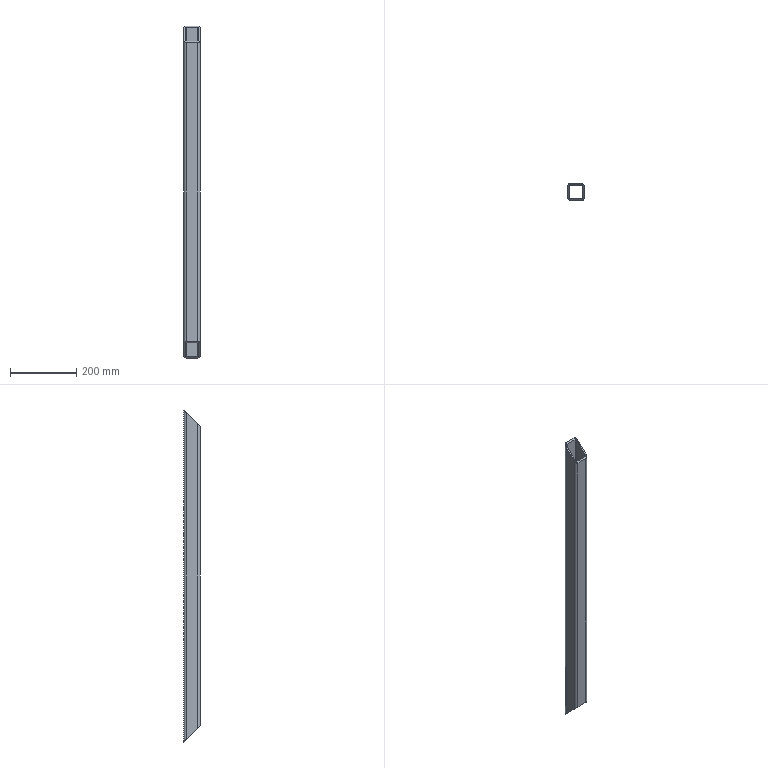Part | SolidWorks | features Extrusion 1, ICE 1, MirrorPattern 1 | 1 solid | 18 faces | box 50 x 50 x 1000 mm | volume 660057 mm3 | plane 10 | cylinder 8 | commonest cylinder face diameters 8 x4 16 x4
STEP:
#1=CARTESIAN_POINT('',(17.,-25.,450.));
#2=VERTEX_POINT('',#1);
#3=CARTESIAN_POINT('',(25.,-17.,458.));
#4=VERTEX_POINT('',#3);
#5=CARTESIAN_POINT('',(17.,-25.,450.));
#6=CARTESIAN_POINT('',(21.686,-25.,450.));
#7=CARTESIAN_POINT('',(25.,-21.686,453.314));
#8=CARTESIAN_POINT('',(25.,-17.,458.));
#9=(BOUNDED_CURVE()B_SPLINE_CURVE(3,(#5,#6,#7,#8),.UNSPECIFIED.,.F.,.T.)B_SPLINE_CURVE_WITH_KNOTS((4,4),(0.,1.571),.UNSPECIFIED.)CURVE()GEOMETRIC_REPRESENTATION_ITEM()RATIONAL_B_SPLINE_CURVE((1.,0.8047,0.8047,1.))REPRESENTATION_ITEM(''));
#10=EDGE_CURVE('',#2,#4,#9,.T.);
#11=ORIENTED_EDGE('',*,*,#10,.F.);
#12=CARTESIAN_POINT('',(17.,-25.,-450.));
#13=VERTEX_POINT('',#12);
#14=CARTESIAN_POINT('',(17.,-25.,500.));
#15=DIRECTION('',(0.,0.,-1.));
#16=VECTOR('',#15,1000.);
#17=LINE('',#14,#16);
#18=EDGE_CURVE('',#2,#13,#17,.T.);
#19=ORIENTED_EDGE('',*,*,#18,.T.);
#20=CARTESIAN_POINT('',(25.,-17.,-458.));
#21=VERTEX_POINT('',#20);
#22=CARTESIAN_POINT('',(17.,-25.,-450.));
#23=CARTESIAN_POINT('',(21.686,-25.,-450.));
#24=CARTESIAN_POINT('',(25.,-21.686,-453.314));
#25=CARTESIAN_POINT('',(25.,-17.,-458.));
#26=(BOUNDED_CURVE()B_SPLINE_CURVE(3,(#22,#23,#24,#25),.UNSPECIFIED.,.F.,.T.)B_SPLINE_CURVE_WITH_KNOTS((4,4),(3.142,4.712),.UNSPECIFIED.)CURVE()GEOMETRIC_REPRESENTATION_ITEM()RATIONAL_B_SPLINE_CURVE((1.,0.8047,0.8047,1.))REPRESENTATION_ITEM(''));
#27=EDGE_CURVE('',#13,#21,#26,.T.);
#28=ORIENTED_EDGE('',*,*,#27,.T.);
#29=CARTESIAN_POINT('',(25.,-17.,500.));
#30=DIRECTION('',(0.,0.,-1.));
#31=VECTOR('',#30,1000.);
#32=LINE('',#29,#31);
#33=EDGE_CURVE('',#4,#21,#32,.T.);
#34=ORIENTED_EDGE('',*,*,#33,.F.);
#35=EDGE_LOOP('',(#11,#19,#28,#34));
#36=FACE_OUTER_BOUND('',#35,.T.);
#37=CARTESIAN_POINT('',(17.,-17.,500.));
#38=DIRECTION('',(0.,0.,-1.));
#39=DIRECTION('',(-1.,0.,0.));
#40=AXIS2_PLACEMENT_3D('',#37,#38,#39);
#41=CYLINDRICAL_SURFACE('',#40,8.);
#42=ADVANCED_FACE('',(#36),#41,.T.);
#43=CARTESIAN_POINT('',(25.,17.,492.));
#44=VERTEX_POINT('',#43);
#45=CARTESIAN_POINT('',(25.,25.,500.));
#46=DIRECTION('',(0.,0.7071,0.7071));
#47=VECTOR('',#46,1000.);
#48=LINE('',#45,#47);
#49=EDGE_CURVE('',#4,#44,#48,.T.);
#50=ORIENTED_EDGE('',*,*,#49,.F.);
#51=ORIENTED_EDGE('',*,*,#33,.T.);
#52=CARTESIAN_POINT('',(25.,17.,-492.));
#53=VERTEX_POINT('',#52);
#54=CARTESIAN_POINT('',(25.,25.,-500.));
#55=DIRECTION('',(0.,0.7071,-0.7071));
#56=VECTOR('',#55,1000.);
#57=LINE('',#54,#56);
#58=EDGE_CURVE('',#21,#53,#57,.T.);
#59=ORIENTED_EDGE('',*,*,#58,.T.);
#60=CARTESIAN_POINT('',(25.,17.,500.));
#61=DIRECTION('',(0.,0.,-1.));
#62=VECTOR('',#61,1000.);
#63=LINE('',#60,#62);
#64=EDGE_CURVE('',#44,#53,#63,.T.);
#65=ORIENTED_EDGE('',*,*,#64,.F.);
#66=EDGE_LOOP('',(#50,#51,#59,#65));
#67=FACE_OUTER_BOUND('',#66,.T.);
#68=CARTESIAN_POINT('',(25.,-17.,500.));
#69=DIRECTION('',(-1.,0.,0.));
#70=DIRECTION('',(0.,0.,1.));
#71=AXIS2_PLACEMENT_3D('',#68,#69,#70);
#72=PLANE('',#71);
#73=ADVANCED_FACE('',(#67),#72,.F.);
#74=CARTESIAN_POINT('',(17.,25.,500.));
#75=VERTEX_POINT('',#74);
#76=CARTESIAN_POINT('',(25.,17.,492.));
#77=CARTESIAN_POINT('',(25.,21.686,496.686));
#78=CARTESIAN_POINT('',(21.686,25.,500.));
#79=CARTESIAN_POINT('',(17.,25.,500.));
#80=(BOUNDED_CURVE()B_SPLINE_CURVE(3,(#76,#77,#78,#79),.UNSPECIFIED.,.F.,.T.)B_SPLINE_CURVE_WITH_KNOTS((4,4),(1.571,3.142),.UNSPECIFIED.)CURVE()GEOMETRIC_REPRESENTATION_ITEM()RATIONAL_B_SPLINE_CURVE((1.,0.8047,0.8047,1.))REPRESENTATION_ITEM(''));
#81=EDGE_CURVE('',#44,#75,#80,.T.);
#82=ORIENTED_EDGE('',*,*,#81,.F.);
#83=ORIENTED_EDGE('',*,*,#64,.T.);
#84=CARTESIAN_POINT('',(17.,25.,-500.));
#85=VERTEX_POINT('',#84);
#86=CARTESIAN_POINT('',(25.,17.,-492.));
#87=CARTESIAN_POINT('',(25.,21.686,-496.686));
#88=CARTESIAN_POINT('',(21.686,25.,-500.));
#89=CARTESIAN_POINT('',(17.,25.,-500.));
#90=(BOUNDED_CURVE()B_SPLINE_CURVE(3,(#86,#87,#88,#89),.UNSPECIFIED.,.F.,.T.)B_SPLINE_CURVE_WITH_KNOTS((4,4),(4.712,6.283),.UNSPECIFIED.)CURVE()GEOMETRIC_REPRESENTATION_ITEM()RATIONAL_B_SPLINE_CURVE((1.,0.8047,0.8047,1.))REPRESENTATION_ITEM(''));
#91=EDGE_CURVE('',#53,#85,#90,.T.);
#92=ORIENTED_EDGE('',*,*,#91,.T.);
#93=CARTESIAN_POINT('',(17.,25.,500.));
#94=DIRECTION('',(0.,0.,-1.));
#95=VECTOR('',#94,1000.);
#96=LINE('',#93,#95);
#97=EDGE_CURVE('',#75,#85,#96,.T.);
#98=ORIENTED_EDGE('',*,*,#97,.F.);
#99=EDGE_LOOP('',(#82,#83,#92,#98));
#100=FACE_OUTER_BOUND('',#99,.T.);
#101=CARTESIAN_POINT('',(17.,17.,500.));
#102=DIRECTION('',(0.,0.,-1.));
#103=DIRECTION('',(-1.,0.,0.));
#104=AXIS2_PLACEMENT_3D('',#101,#102,#103);
#105=CYLINDRICAL_SURFACE('',#104,8.);
#106=ADVANCED_FACE('',(#100),#105,.T.);
#107=CARTESIAN_POINT('',(-17.,25.,500.));
#108=VERTEX_POINT('',#107);
#109=CARTESIAN_POINT('',(-25.,17.,492.));
#110=VERTEX_POINT('',#109);
#111=CARTESIAN_POINT('',(-17.,25.,500.));
#112=CARTESIAN_POINT('',(-21.686,25.,500.));
#113=CARTESIAN_POINT('',(-25.,21.686,496.686));
#114=CARTESIAN_POINT('',(-25.,17.,492.));
#115=(BOUNDED_CURVE()B_SPLINE_CURVE(3,(#111,#112,#113,#114),.UNSPECIFIED.,.F.,.T.)B_SPLINE_CURVE_WITH_KNOTS((4,4),(3.142,4.712),.UNSPECIFIED.)CURVE()GEOMETRIC_REPRESENTATION_ITEM()RATIONAL_B_SPLINE_CURVE((1.,0.8047,0.8047,1.))REPRESENTATION_ITEM(''));
#116=EDGE_CURVE('',#108,#110,#115,.T.);
#117=ORIENTED_EDGE('',*,*,#116,.F.);
#118=CARTESIAN_POINT('',(-17.,25.,-500.));
#119=VERTEX_POINT('',#118);
#120=CARTESIAN_POINT('',(-17.,25.,500.));
#121=DIRECTION('',(0.,0.,-1.));
#122=VECTOR('',#121,1000.);
#123=LINE('',#120,#122);
#124=EDGE_CURVE('',#108,#119,#123,.T.);
#125=ORIENTED_EDGE('',*,*,#124,.T.);
#126=CARTESIAN_POINT('',(-25.,17.,-492.));
#127=VERTEX_POINT('',#126);
#128=CARTESIAN_POINT('',(-17.,25.,-500.));
#129=CARTESIAN_POINT('',(-21.686,25.,-500.));
#130=CARTESIAN_POINT('',(-25.,21.686,-496.686));
#131=CARTESIAN_POINT('',(-25.,17.,-492.));
#132=(BOUNDED_CURVE()B_SPLINE_CURVE(3,(#128,#129,#130,#131),.UNSPECIFIED.,.F.,.F.)B_SPLINE_CURVE_WITH_KNOTS((4,4),(0.,1.571),.UNSPECIFIED.)CURVE()GEOMETRIC_REPRESENTATION_ITEM()RATIONAL_B_SPLINE_CURVE((1.,0.8047,0.8047,1.))REPRESENTATION_ITEM(''));
#133=EDGE_CURVE('',#119,#127,#132,.T.);
#134=ORIENTED_EDGE('',*,*,#133,.T.);
#135=CARTESIAN_POINT('',(-25.,17.,500.));
#136=DIRECTION('',(0.,0.,-1.));
#137=VECTOR('',#136,1000.);
#138=LINE('',#135,#137);
#139=EDGE_CURVE('',#110,#127,#138,.T.);
#140=ORIENTED_EDGE('',*,*,#139,.F.);
#141=EDGE_LOOP('',(#117,#125,#134,#140));
#142=FACE_OUTER_BOUND('',#141,.T.);
#143=CARTESIAN_POINT('',(-17.,17.,500.));
#144=DIRECTION('',(0.,0.,-1.));
#145=DIRECTION('',(-1.,0.,0.));
#146=AXIS2_PLACEMENT_3D('',#143,#144,#145);
#147=CYLINDRICAL_SURFACE('',#146,8.);
#148=ADVANCED_FACE('',(#142),#147,.T.);
#149=CARTESIAN_POINT('',(-25.,-17.,458.));
#150=VERTEX_POINT('',#149);
#151=CARTESIAN_POINT('',(-25.,25.,500.));
#152=DIRECTION('',(0.,0.7071,0.7071));
#153=VECTOR('',#152,1000.);
#154=LINE('',#151,#153);
#155=EDGE_CURVE('',#150,#110,#154,.T.);
#156=ORIENTED_EDGE('',*,*,#155,.T.);
#157=ORIENTED_EDGE('',*,*,#139,.T.);
#158=CARTESIAN_POINT('',(-25.,-17.,-458.));
#159=VERTEX_POINT('',#158);
#160=CARTESIAN_POINT('',(-25.,25.,-500.));
#161=DIRECTION('',(0.,0.7071,-0.7071));
#162=VECTOR('',#161,1000.);
#163=LINE('',#160,#162);
#164=EDGE_CURVE('',#159,#127,#163,.T.);
#165=ORIENTED_EDGE('',*,*,#164,.F.);
#166=CARTESIAN_POINT('',(-25.,-17.,500.));
#167=DIRECTION('',(0.,0.,-1.));
#168=VECTOR('',#167,1000.);
#169=LINE('',#166,#168);
#170=EDGE_CURVE('',#150,#159,#169,.T.);
#171=ORIENTED_EDGE('',*,*,#170,.F.);
#172=EDGE_LOOP('',(#156,#157,#165,#171));
#173=FACE_OUTER_BOUND('',#172,.T.);
#174=CARTESIAN_POINT('',(-25.,-17.,500.));
#175=DIRECTION('',(1.,0.,0.));
#176=DIRECTION('',(0.,0.,-1.));
#177=AXIS2_PLACEMENT_3D('',#174,#175,#176);
#178=PLANE('',#177);
#179=ADVANCED_FACE('',(#173),#178,.F.);
#180=CARTESIAN_POINT('',(-17.,-25.,450.));
#181=VERTEX_POINT('',#180);
#182=CARTESIAN_POINT('',(-25.,-17.,458.));
#183=CARTESIAN_POINT('',(-25.,-21.686,453.314));
#184=CARTESIAN_POINT('',(-21.686,-25.,450.));
#185=CARTESIAN_POINT('',(-17.,-25.,450.));
#186=(BOUNDED_CURVE()B_SPLINE_CURVE(3,(#182,#183,#184,#185),.UNSPECIFIED.,.F.,.T.)B_SPLINE_CURVE_WITH_KNOTS((4,4),(4.712,6.283),.UNSPECIFIED.)CURVE()GEOMETRIC_REPRESENTATION_ITEM()RATIONAL_B_SPLINE_CURVE((1.,0.8047,0.8047,1.))REPRESENTATION_ITEM(''));
#187=EDGE_CURVE('',#150,#181,#186,.T.);
#188=ORIENTED_EDGE('',*,*,#187,.F.);
#189=ORIENTED_EDGE('',*,*,#170,.T.);
#190=CARTESIAN_POINT('',(-17.,-25.,-450.));
#191=VERTEX_POINT('',#190);
#192=CARTESIAN_POINT('',(-25.,-17.,-458.));
#193=CARTESIAN_POINT('',(-25.,-21.686,-453.314));
#194=CARTESIAN_POINT('',(-21.686,-25.,-450.));
#195=CARTESIAN_POINT('',(-17.,-25.,-450.));
#196=(BOUNDED_CURVE()B_SPLINE_CURVE(3,(#192,#193,#194,#195),.UNSPECIFIED.,.F.,.T.)B_SPLINE_CURVE_WITH_KNOTS((4,4),(1.571,3.142),.UNSPECIFIED.)CURVE()GEOMETRIC_REPRESENTATION_ITEM()RATIONAL_B_SPLINE_CURVE((1.,0.8047,0.8047,1.))REPRESENTATION_ITEM(''));
#197=EDGE_CURVE('',#159,#191,#196,.T.);
#198=ORIENTED_EDGE('',*,*,#197,.T.);
#199=CARTESIAN_POINT('',(-17.,-25.,500.));
#200=DIRECTION('',(0.,0.,-1.));
#201=VECTOR('',#200,1000.);
#202=LINE('',#199,#201);
#203=EDGE_CURVE('',#181,#191,#202,.T.);
#204=ORIENTED_EDGE('',*,*,#203,.F.);
#205=EDGE_LOOP('',(#188,#189,#198,#204));
#206=FACE_OUTER_BOUND('',#205,.T.);
#207=CARTESIAN_POINT('',(-17.,-17.,500.));
#208=DIRECTION('',(0.,0.,-1.));
#209=DIRECTION('',(-1.,0.,0.));
#210=AXIS2_PLACEMENT_3D('',#207,#208,#209);
#211=CYLINDRICAL_SURFACE('',#210,8.);
#212=ADVANCED_FACE('',(#206),#211,.T.);
#213=CARTESIAN_POINT('',(25.,-25.,450.));
#214=DIRECTION('',(-1.,0.,0.));
#215=VECTOR('',#214,1000.);
#216=LINE('',#213,#215);
#217=EDGE_CURVE('',#2,#181,#216,.T.);
#218=ORIENTED_EDGE('',*,*,#217,.T.);
#219=ORIENTED_EDGE('',*,*,#203,.T.);
#220=CARTESIAN_POINT('',(25.,-25.,-450.));
#221=DIRECTION('',(-1.,0.,0.));
#222=VECTOR('',#221,1000.);
#223=LINE('',#220,#222);
#224=EDGE_CURVE('',#13,#191,#223,.T.);
#225=ORIENTED_EDGE('',*,*,#224,.F.);
#226=ORIENTED_EDGE('',*,*,#18,.F.);
#227=EDGE_LOOP('',(#218,#219,#225,#226));
#228=FACE_OUTER_BOUND('',#227,.T.);
#229=CARTESIAN_POINT('',(-17.,-25.,500.));
#230=DIRECTION('',(0.,1.,0.));
#231=DIRECTION('',(0.,0.,1.));
#232=AXIS2_PLACEMENT_3D('',#229,#230,#231);
#233=PLANE('',#232);
#234=ADVANCED_FACE('',(#228),#233,.F.);
#235=CARTESIAN_POINT('',(-17.,21.,496.));
#236=VERTEX_POINT('',#235);
#237=CARTESIAN_POINT('',(-17.,21.,-496.));
#238=VERTEX_POINT('',#237);
#239=CARTESIAN_POINT('',(-17.,21.,500.));
#240=DIRECTION('',(0.,0.,-1.));
#241=VECTOR('',#240,1000.);
#242=LINE('',#239,#241);
#243=EDGE_CURVE('',#236,#238,#242,.T.);
#244=ORIENTED_EDGE('',*,*,#243,.F.);
#245=CARTESIAN_POINT('',(-21.,17.,492.));
#246=VERTEX_POINT('',#245);
#247=CARTESIAN_POINT('',(-17.,21.,496.));
#248=CARTESIAN_POINT('',(-19.343,21.,496.));
#249=CARTESIAN_POINT('',(-21.,19.343,494.343));
#250=CARTESIAN_POINT('',(-21.,17.,492.));
#251=(BOUNDED_CURVE()B_SPLINE_CURVE(3,(#247,#248,#249,#250),.UNSPECIFIED.,.F.,.T.)B_SPLINE_CURVE_WITH_KNOTS((4,4),(3.142,4.712),.UNSPECIFIED.)CURVE()GEOMETRIC_REPRESENTATION_ITEM()RATIONAL_B_SPLINE_CURVE((1.,0.8047,0.8047,1.))REPRESENTATION_ITEM(''));
#252=EDGE_CURVE('',#236,#246,#251,.T.);
#253=ORIENTED_EDGE('',*,*,#252,.T.);
#254=CARTESIAN_POINT('',(-21.,17.,-492.));
#255=VERTEX_POINT('',#254);
#256=CARTESIAN_POINT('',(-21.,17.,500.));
#257=DIRECTION('',(0.,0.,-1.));
#258=VECTOR('',#257,1000.);
#259=LINE('',#256,#258);
#260=EDGE_CURVE('',#246,#255,#259,.T.);
#261=ORIENTED_EDGE('',*,*,#260,.T.);
#262=CARTESIAN_POINT('',(-17.,21.,-496.));
#263=CARTESIAN_POINT('',(-19.343,21.,-496.));
#264=CARTESIAN_POINT('',(-21.,19.343,-494.343));
#265=CARTESIAN_POINT('',(-21.,17.,-492.));
#266=(BOUNDED_CURVE()B_SPLINE_CURVE(3,(#262,#263,#264,#265),.UNSPECIFIED.,.F.,.T.)B_SPLINE_CURVE_WITH_KNOTS((4,4),(0.,1.571),.UNSPECIFIED.)CURVE()GEOMETRIC_REPRESENTATION_ITEM()RATIONAL_B_SPLINE_CURVE((1.,0.8047,0.8047,1.))REPRESENTATION_ITEM(''));
#267=EDGE_CURVE('',#238,#255,#266,.T.);
#268=ORIENTED_EDGE('',*,*,#267,.F.);
#269=EDGE_LOOP('',(#244,#253,#261,#268));
#270=FACE_OUTER_BOUND('',#269,.T.);
#271=CARTESIAN_POINT('',(-17.,17.,500.));
#272=DIRECTION('',(0.,0.,-1.));
#273=DIRECTION('',(-1.,0.,0.));
#274=AXIS2_PLACEMENT_3D('',#271,#272,#273);
#275=CYLINDRICAL_SURFACE('',#274,4.);
#276=ADVANCED_FACE('',(#270),#275,.F.);
#277=ORIENTED_EDGE('',*,*,#260,.F.);
#278=CARTESIAN_POINT('',(-21.,-17.,458.));
#279=VERTEX_POINT('',#278);
#280=CARTESIAN_POINT('',(-21.,4.,479.));
#281=DIRECTION('',(0.,-0.7071,-0.7071));
#282=VECTOR('',#281,1000.);
#283=LINE('',#280,#282);
#284=EDGE_CURVE('',#246,#279,#283,.T.);
#285=ORIENTED_EDGE('',*,*,#284,.T.);
#286=CARTESIAN_POINT('',(-21.,-17.,-458.));
#287=VERTEX_POINT('',#286);
#288=CARTESIAN_POINT('',(-21.,-17.,500.));
#289=DIRECTION('',(0.,0.,-1.));
#290=VECTOR('',#289,1000.);
#291=LINE('',#288,#290);
#292=EDGE_CURVE('',#279,#287,#291,.T.);
#293=ORIENTED_EDGE('',*,*,#292,.T.);
#294=CARTESIAN_POINT('',(-21.,-496.,21.));
#295=DIRECTION('',(0.,-0.7071,0.7071));
#296=VECTOR('',#295,1000.);
#297=LINE('',#294,#296);
#298=EDGE_CURVE('',#255,#287,#297,.T.);
#299=ORIENTED_EDGE('',*,*,#298,.F.);
#300=EDGE_LOOP('',(#277,#285,#293,#299));
#301=FACE_OUTER_BOUND('',#300,.T.);
#302=CARTESIAN_POINT('',(-21.,-17.,500.));
#303=DIRECTION('',(1.,0.,0.));
#304=DIRECTION('',(0.,0.,-1.));
#305=AXIS2_PLACEMENT_3D('',#302,#303,#304);
#306=PLANE('',#305);
#307=ADVANCED_FACE('',(#301),#306,.T.);
#308=ORIENTED_EDGE('',*,*,#292,.F.);
#309=CARTESIAN_POINT('',(-17.,-21.,454.));
#310=VERTEX_POINT('',#309);
#311=CARTESIAN_POINT('',(-21.,-17.,458.));
#312=CARTESIAN_POINT('',(-21.,-19.343,455.657));
#313=CARTESIAN_POINT('',(-19.343,-21.,454.));
#314=CARTESIAN_POINT('',(-17.,-21.,454.));
#315=(BOUNDED_CURVE()B_SPLINE_CURVE(3,(#311,#312,#313,#314),.UNSPECIFIED.,.F.,.T.)B_SPLINE_CURVE_WITH_KNOTS((4,4),(4.712,6.283),.UNSPECIFIED.)CURVE()GEOMETRIC_REPRESENTATION_ITEM()RATIONAL_B_SPLINE_CURVE((1.,0.8047,0.8047,1.))REPRESENTATION_ITEM(''));
#316=EDGE_CURVE('',#279,#310,#315,.T.);
#317=ORIENTED_EDGE('',*,*,#316,.T.);
#318=CARTESIAN_POINT('',(-17.,-21.,-454.));
#319=VERTEX_POINT('',#318);
#320=CARTESIAN_POINT('',(-17.,-21.,500.));
#321=DIRECTION('',(0.,0.,-1.));
#322=VECTOR('',#321,1000.);
#323=LINE('',#320,#322);
#324=EDGE_CURVE('',#310,#319,#323,.T.);
#325=ORIENTED_EDGE('',*,*,#324,.T.);
#326=CARTESIAN_POINT('',(-21.,-17.,-458.));
#327=CARTESIAN_POINT('',(-21.,-19.343,-455.657));
#328=CARTESIAN_POINT('',(-19.343,-21.,-454.));
#329=CARTESIAN_POINT('',(-17.,-21.,-454.));
#330=(BOUNDED_CURVE()B_SPLINE_CURVE(3,(#326,#327,#328,#329),.UNSPECIFIED.,.F.,.T.)B_SPLINE_CURVE_WITH_KNOTS((4,4),(1.571,3.142),.UNSPECIFIED.)CURVE()GEOMETRIC_REPRESENTATION_ITEM()RATIONAL_B_SPLINE_CURVE((1.,0.8047,0.8047,1.))REPRESENTATION_ITEM(''));
#331=EDGE_CURVE('',#287,#319,#330,.T.);
#332=ORIENTED_EDGE('',*,*,#331,.F.);
#333=EDGE_LOOP('',(#308,#317,#325,#332));
#334=FACE_OUTER_BOUND('',#333,.T.);
#335=CARTESIAN_POINT('',(-17.,-17.,500.));
#336=DIRECTION('',(0.,0.,-1.));
#337=DIRECTION('',(-1.,0.,0.));
#338=AXIS2_PLACEMENT_3D('',#335,#336,#337);
#339=CYLINDRICAL_SURFACE('',#338,4.);
#340=ADVANCED_FACE('',(#334),#339,.F.);
#341=ORIENTED_EDGE('',*,*,#324,.F.);
#342=CARTESIAN_POINT('',(17.,-21.,454.));
#343=VERTEX_POINT('',#342);
#344=CARTESIAN_POINT('',(-17.,-21.,454.));
#345=DIRECTION('',(1.,0.,0.));
#346=VECTOR('',#345,1000.);
#347=LINE('',#344,#346);
#348=EDGE_CURVE('',#310,#343,#347,.T.);
#349=ORIENTED_EDGE('',*,*,#348,.T.);
#350=CARTESIAN_POINT('',(17.,-21.,-454.));
#351=VERTEX_POINT('',#350);
#352=CARTESIAN_POINT('',(17.,-21.,500.));
#353=DIRECTION('',(0.,0.,-1.));
#354=VECTOR('',#353,1000.);
#355=LINE('',#352,#354);
#356=EDGE_CURVE('',#343,#351,#355,.T.);
#357=ORIENTED_EDGE('',*,*,#356,.T.);
#358=CARTESIAN_POINT('',(-17.,-21.,-454.));
#359=DIRECTION('',(1.,0.,0.));
#360=VECTOR('',#359,1000.);
#361=LINE('',#358,#360);
#362=EDGE_CURVE('',#319,#351,#361,.T.);
#363=ORIENTED_EDGE('',*,*,#362,.F.);
#364=EDGE_LOOP('',(#341,#349,#357,#363));
#365=FACE_OUTER_BOUND('',#364,.T.);
#366=CARTESIAN_POINT('',(-17.,-21.,500.));
#367=DIRECTION('',(0.,1.,0.));
#368=DIRECTION('',(0.,0.,1.));
#369=AXIS2_PLACEMENT_3D('',#366,#367,#368);
#370=PLANE('',#369);
#371=ADVANCED_FACE('',(#365),#370,.T.);
#372=ORIENTED_EDGE('',*,*,#356,.F.);
#373=CARTESIAN_POINT('',(21.,-17.,458.));
#374=VERTEX_POINT('',#373);
#375=CARTESIAN_POINT('',(17.,-21.,454.));
#376=CARTESIAN_POINT('',(19.343,-21.,454.));
#377=CARTESIAN_POINT('',(21.,-19.343,455.657));
#378=CARTESIAN_POINT('',(21.,-17.,458.));
#379=(BOUNDED_CURVE()B_SPLINE_CURVE(3,(#375,#376,#377,#378),.UNSPECIFIED.,.F.,.F.)B_SPLINE_CURVE_WITH_KNOTS((4,4),(0.,1.571),.UNSPECIFIED.)CURVE()GEOMETRIC_REPRESENTATION_ITEM()RATIONAL_B_SPLINE_CURVE((1.,0.8047,0.8047,1.))REPRESENTATION_ITEM(''));
#380=EDGE_CURVE('',#343,#374,#379,.T.);
#381=ORIENTED_EDGE('',*,*,#380,.T.);
#382=CARTESIAN_POINT('',(21.,-17.,-458.));
#383=VERTEX_POINT('',#382);
#384=CARTESIAN_POINT('',(21.,-17.,500.));
#385=DIRECTION('',(0.,0.,-1.));
#386=VECTOR('',#385,1000.);
#387=LINE('',#384,#386);
#388=EDGE_CURVE('',#374,#383,#387,.T.);
#389=ORIENTED_EDGE('',*,*,#388,.T.);
#390=CARTESIAN_POINT('',(17.,-21.,-454.));
#391=CARTESIAN_POINT('',(19.343,-21.,-454.));
#392=CARTESIAN_POINT('',(21.,-19.343,-455.657));
#393=CARTESIAN_POINT('',(21.,-17.,-458.));
#394=(BOUNDED_CURVE()B_SPLINE_CURVE(3,(#390,#391,#392,#393),.UNSPECIFIED.,.F.,.T.)B_SPLINE_CURVE_WITH_KNOTS((4,4),(3.142,4.712),.UNSPECIFIED.)CURVE()GEOMETRIC_REPRESENTATION_ITEM()RATIONAL_B_SPLINE_CURVE((1.,0.8047,0.8047,1.))REPRESENTATION_ITEM(''));
#395=EDGE_CURVE('',#351,#383,#394,.T.);
#396=ORIENTED_EDGE('',*,*,#395,.F.);
#397=EDGE_LOOP('',(#372,#381,#389,#396));
#398=FACE_OUTER_BOUND('',#397,.T.);
#399=CARTESIAN_POINT('',(17.,-17.,500.));
#400=DIRECTION('',(0.,0.,-1.));
#401=DIRECTION('',(-1.,0.,0.));
#402=AXIS2_PLACEMENT_3D('',#399,#400,#401);
#403=CYLINDRICAL_SURFACE('',#402,4.);
#404=ADVANCED_FACE('',(#398),#403,.F.);
#405=ORIENTED_EDGE('',*,*,#388,.F.);
#406=CARTESIAN_POINT('',(21.,17.,492.));
#407=VERTEX_POINT('',#406);
#408=CARTESIAN_POINT('',(21.,4.,479.));
#409=DIRECTION('',(0.,0.7071,0.7071));
#410=VECTOR('',#409,1000.);
#411=LINE('',#408,#410);
#412=EDGE_CURVE('',#374,#407,#411,.T.);
#413=ORIENTED_EDGE('',*,*,#412,.T.);
#414=CARTESIAN_POINT('',(21.,17.,-492.));
#415=VERTEX_POINT('',#414);
#416=CARTESIAN_POINT('',(21.,17.,500.));
#417=DIRECTION('',(0.,0.,-1.));
#418=VECTOR('',#417,1000.);
#419=LINE('',#416,#418);
#420=EDGE_CURVE('',#407,#415,#419,.T.);
#421=ORIENTED_EDGE('',*,*,#420,.T.);
#422=CARTESIAN_POINT('',(21.,-496.,21.));
#423=DIRECTION('',(0.,0.7071,-0.7071));
#424=VECTOR('',#423,1000.);
#425=LINE('',#422,#424);
#426=EDGE_CURVE('',#383,#415,#425,.T.);
#427=ORIENTED_EDGE('',*,*,#426,.F.);
#428=EDGE_LOOP('',(#405,#413,#421,#427));
#429=FACE_OUTER_BOUND('',#428,.T.);
#430=CARTESIAN_POINT('',(21.,-17.,500.));
#431=DIRECTION('',(-1.,0.,0.));
#432=DIRECTION('',(0.,0.,1.));
#433=AXIS2_PLACEMENT_3D('',#430,#431,#432);
#434=PLANE('',#433);
#435=ADVANCED_FACE('',(#429),#434,.T.);
#436=ORIENTED_EDGE('',*,*,#420,.F.);
#437=CARTESIAN_POINT('',(17.,21.,496.));
#438=VERTEX_POINT('',#437);
#439=CARTESIAN_POINT('',(21.,17.,492.));
#440=CARTESIAN_POINT('',(21.,19.343,494.343));
#441=CARTESIAN_POINT('',(19.343,21.,496.));
#442=CARTESIAN_POINT('',(17.,21.,496.));
#443=(BOUNDED_CURVE()B_SPLINE_CURVE(3,(#439,#440,#441,#442),.UNSPECIFIED.,.F.,.T.)B_SPLINE_CURVE_WITH_KNOTS((4,4),(1.571,3.142),.UNSPECIFIED.)CURVE()GEOMETRIC_REPRESENTATION_ITEM()RATIONAL_B_SPLINE_CURVE((1.,0.8047,0.8047,1.))REPRESENTATION_ITEM(''));
#444=EDGE_CURVE('',#407,#438,#443,.T.);
#445=ORIENTED_EDGE('',*,*,#444,.T.);
#446=CARTESIAN_POINT('',(17.,21.,-496.));
#447=VERTEX_POINT('',#446);
#448=CARTESIAN_POINT('',(17.,21.,500.));
#449=DIRECTION('',(0.,0.,-1.));
#450=VECTOR('',#449,1000.);
#451=LINE('',#448,#450);
#452=EDGE_CURVE('',#438,#447,#451,.T.);
#453=ORIENTED_EDGE('',*,*,#452,.T.);
#454=CARTESIAN_POINT('',(21.,17.,-492.));
#455=CARTESIAN_POINT('',(21.,19.343,-494.343));
#456=CARTESIAN_POINT('',(19.343,21.,-496.));
#457=CARTESIAN_POINT('',(17.,21.,-496.));
#458=(BOUNDED_CURVE()B_SPLINE_CURVE(3,(#454,#455,#456,#457),.UNSPECIFIED.,.F.,.T.)B_SPLINE_CURVE_WITH_KNOTS((4,4),(4.712,6.283),.UNSPECIFIED.)CURVE()GEOMETRIC_REPRESENTATION_ITEM()RATIONAL_B_SPLINE_CURVE((1.,0.8047,0.8047,1.))REPRESENTATION_ITEM(''));
#459=EDGE_CURVE('',#415,#447,#458,.T.);
#460=ORIENTED_EDGE('',*,*,#459,.F.);
#461=EDGE_LOOP('',(#436,#445,#453,#460));
#462=FACE_OUTER_BOUND('',#461,.T.);
#463=CARTESIAN_POINT('',(17.,17.,500.));
#464=DIRECTION('',(0.,0.,-1.));
#465=DIRECTION('',(-1.,0.,0.));
#466=AXIS2_PLACEMENT_3D('',#463,#464,#465);
#467=CYLINDRICAL_SURFACE('',#466,4.);
#468=ADVANCED_FACE('',(#462),#467,.F.);
#469=ORIENTED_EDGE('',*,*,#452,.F.);
#470=CARTESIAN_POINT('',(-17.,21.,496.));
#471=DIRECTION('',(-1.,0.,0.));
#472=VECTOR('',#471,1000.);
#473=LINE('',#470,#472);
#474=EDGE_CURVE('',#438,#236,#473,.T.);
#475=ORIENTED_EDGE('',*,*,#474,.T.);
#476=ORIENTED_EDGE('',*,*,#243,.T.);
#477=CARTESIAN_POINT('',(-17.,21.,-496.));
#478=DIRECTION('',(-1.,0.,0.));
#479=VECTOR('',#478,1000.);
#480=LINE('',#477,#479);
#481=EDGE_CURVE('',#447,#238,#480,.T.);
#482=ORIENTED_EDGE('',*,*,#481,.F.);
#483=EDGE_LOOP('',(#469,#475,#476,#482));
#484=FACE_OUTER_BOUND('',#483,.T.);
#485=CARTESIAN_POINT('',(-17.,21.,500.));
#486=DIRECTION('',(0.,-1.,0.));
#487=DIRECTION('',(0.,0.,-1.));
#488=AXIS2_PLACEMENT_3D('',#485,#486,#487);
#489=PLANE('',#488);
#490=ADVANCED_FACE('',(#484),#489,.T.);
#491=CARTESIAN_POINT('',(-17.,25.,-500.));
#492=DIRECTION('',(-1.,0.,0.));
#493=VECTOR('',#492,1000.);
#494=LINE('',#491,#493);
#495=EDGE_CURVE('',#85,#119,#494,.T.);
#496=ORIENTED_EDGE('',*,*,#495,.T.);
#497=ORIENTED_EDGE('',*,*,#124,.F.);
#498=CARTESIAN_POINT('',(-17.,25.,500.));
#499=DIRECTION('',(-1.,0.,0.));
#500=VECTOR('',#499,1000.);
#501=LINE('',#498,#500);
#502=EDGE_CURVE('',#75,#108,#501,.T.);
#503=ORIENTED_EDGE('',*,*,#502,.F.);
#504=ORIENTED_EDGE('',*,*,#97,.T.);
#505=EDGE_LOOP('',(#496,#497,#503,#504));
#506=FACE_OUTER_BOUND('',#505,.T.);
#507=CARTESIAN_POINT('',(-17.,25.,500.));
#508=DIRECTION('',(0.,-1.,0.));
#509=DIRECTION('',(0.,0.,-1.));
#510=AXIS2_PLACEMENT_3D('',#507,#508,#509);
#511=PLANE('',#510);
#512=ADVANCED_FACE('',(#506),#511,.F.);
#513=ORIENTED_EDGE('',*,*,#267,.T.);
#514=ORIENTED_EDGE('',*,*,#298,.T.);
#515=ORIENTED_EDGE('',*,*,#331,.T.);
#516=ORIENTED_EDGE('',*,*,#362,.T.);
#517=ORIENTED_EDGE('',*,*,#395,.T.);
#518=ORIENTED_EDGE('',*,*,#426,.T.);
#519=ORIENTED_EDGE('',*,*,#459,.T.);
#520=ORIENTED_EDGE('',*,*,#481,.T.);
#521=EDGE_LOOP('',(#513,#514,#515,#516,#517,#518,#519,#520));
#522=FACE_BOUND('',#521,.T.);
#523=ORIENTED_EDGE('',*,*,#224,.T.);
#524=ORIENTED_EDGE('',*,*,#197,.F.);
#525=ORIENTED_EDGE('',*,*,#164,.T.);
#526=ORIENTED_EDGE('',*,*,#133,.F.);
#527=ORIENTED_EDGE('',*,*,#495,.F.);
#528=ORIENTED_EDGE('',*,*,#91,.F.);
#529=ORIENTED_EDGE('',*,*,#58,.F.);
#530=ORIENTED_EDGE('',*,*,#27,.F.);
#531=EDGE_LOOP('',(#523,#524,#525,#526,#527,#528,#529,#530));
#532=FACE_OUTER_BOUND('',#531,.T.);
#533=CARTESIAN_POINT('',(25.,25.,-500.));
#534=DIRECTION('',(0.,0.7071,0.7071));
#535=DIRECTION('',(0.,-0.7071,0.7071));
#536=AXIS2_PLACEMENT_3D('',#533,#534,#535);
#537=PLANE('',#536);
#538=ADVANCED_FACE('',(#522,#532),#537,.F.);
#539=ORIENTED_EDGE('',*,*,#474,.F.);
#540=ORIENTED_EDGE('',*,*,#444,.F.);
#541=ORIENTED_EDGE('',*,*,#412,.F.);
#542=ORIENTED_EDGE('',*,*,#380,.F.);
#543=ORIENTED_EDGE('',*,*,#348,.F.);
#544=ORIENTED_EDGE('',*,*,#316,.F.);
#545=ORIENTED_EDGE('',*,*,#284,.F.);
#546=ORIENTED_EDGE('',*,*,#252,.F.);
#547=EDGE_LOOP('',(#539,#540,#541,#542,#543,#544,#545,#546));
#548=FACE_BOUND('',#547,.T.);
#549=ORIENTED_EDGE('',*,*,#10,.T.);
#550=ORIENTED_EDGE('',*,*,#49,.T.);
#551=ORIENTED_EDGE('',*,*,#81,.T.);
#552=ORIENTED_EDGE('',*,*,#502,.T.);
#553=ORIENTED_EDGE('',*,*,#116,.T.);
#554=ORIENTED_EDGE('',*,*,#155,.F.);
#555=ORIENTED_EDGE('',*,*,#187,.T.);
#556=ORIENTED_EDGE('',*,*,#217,.F.);
#557=EDGE_LOOP('',(#549,#550,#551,#552,#553,#554,#555,#556));
#558=FACE_OUTER_BOUND('',#557,.T.);
#559=CARTESIAN_POINT('',(25.,25.,500.));
#560=DIRECTION('',(0.,-0.7071,0.7071));
#561=DIRECTION('',(0.,-0.7071,-0.7071));
#562=AXIS2_PLACEMENT_3D('',#559,#560,#561);
#563=PLANE('',#562);
#564=ADVANCED_FACE('',(#548,#558),#563,.T.);
#565=CLOSED_SHELL('',(#42,#73,#106,#148,#179,#212,#234,#276,#307,#340,#371,#404,#435,#468,#490,#512,#538,#564));
#566=MANIFOLD_SOLID_BREP('',#565);
#567=CARTESIAN_POINT('',(0.,0.,0.));
#568=DIRECTION('',(0.,0.,1.));
#569=DIRECTION('',(1.,0.,0.));
#570=AXIS2_PLACEMENT_3D('',#567,#568,#569);
#571=(LENGTH_UNIT()NAMED_UNIT(*)SI_UNIT(.MILLI.,.METRE.));
#572=UNCERTAINTY_MEASURE_WITH_UNIT(LENGTH_MEASURE(0.00001),#571,'','');
#573=(NAMED_UNIT(*)PLANE_ANGLE_UNIT()SI_UNIT($,.RADIAN.));
#574=(NAMED_UNIT(*)SI_UNIT($,.STERADIAN.)SOLID_ANGLE_UNIT());
#575=(GEOMETRIC_REPRESENTATION_CONTEXT(3)GLOBAL_UNCERTAINTY_ASSIGNED_CONTEXT((#572))GLOBAL_UNIT_ASSIGNED_CONTEXT((#571,#573,#574))REPRESENTATION_CONTEXT('',''));
#576=ADVANCED_BREP_SHAPE_REPRESENTATION('',(#566,#570),#575);